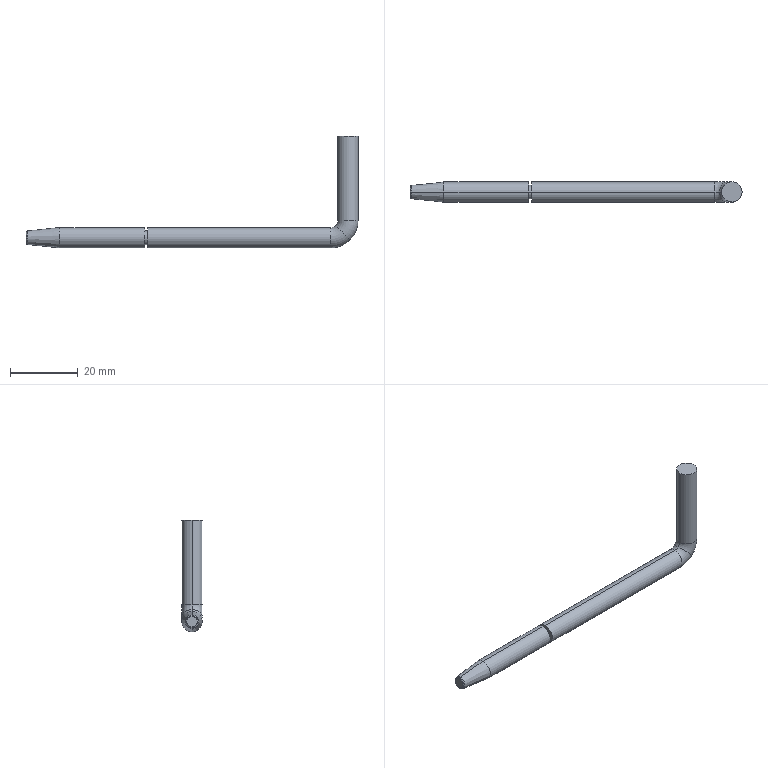Part | NX | features BREP 1 | 1 solid | 22 faces | box 98 x 6 x 33 mm | volume 3371 mm3 | cylinder 8 | torus 8 | plane 4 | cone 2 | commonest cylinder face diameters 6 x6 4 x2
STEP:
#1=CARTESIAN_POINT('',(90.,0.,-3.));
#2=VERTEX_POINT('',#1);
#3=CARTESIAN_POINT('',(35.9,0.,-3.));
#4=VERTEX_POINT('',#3);
#5=CARTESIAN_POINT('',(90.,0.,-3.));
#6=DIRECTION('',(-1.,0.,0.));
#7=VECTOR('',#6,1000.);
#8=LINE('',#5,#7);
#9=EDGE_CURVE('',#2,#4,#8,.T.);
#10=ORIENTED_EDGE('',*,*,#9,.T.);
#11=CARTESIAN_POINT('',(35.9,0.,3.));
#12=VERTEX_POINT('',#11);
#13=CARTESIAN_POINT('',(35.9,0.,0.));
#14=DIRECTION('',(1.,0.,0.));
#15=DIRECTION('',(0.,0.,-1.));
#16=AXIS2_PLACEMENT_3D('',#13,#14,#15);
#17=CIRCLE('',#16,3.);
#18=EDGE_CURVE('',#4,#12,#17,.T.);
#19=ORIENTED_EDGE('',*,*,#18,.T.);
#20=CARTESIAN_POINT('',(90.,0.,3.));
#21=VERTEX_POINT('',#20);
#22=CARTESIAN_POINT('',(90.,0.,3.));
#23=DIRECTION('',(-1.,0.,0.));
#24=VECTOR('',#23,1000.);
#25=LINE('',#22,#24);
#26=EDGE_CURVE('',#21,#12,#25,.T.);
#27=ORIENTED_EDGE('',*,*,#26,.F.);
#28=CARTESIAN_POINT('',(90.,0.,0.));
#29=DIRECTION('',(-1.,0.,0.));
#30=DIRECTION('',(0.,0.,1.));
#31=AXIS2_PLACEMENT_3D('',#28,#29,#30);
#32=CIRCLE('',#31,3.);
#33=EDGE_CURVE('',#21,#2,#32,.T.);
#34=ORIENTED_EDGE('',*,*,#33,.T.);
#35=EDGE_LOOP('',(#10,#19,#27,#34));
#36=FACE_BOUND('',#35,.T.);
#37=CARTESIAN_POINT('',(0.,0.,0.));
#38=DIRECTION('',(1.,0.,0.));
#39=DIRECTION('',(0.,0.,-1.));
#40=AXIS2_PLACEMENT_3D('',#37,#38,#39);
#41=CYLINDRICAL_SURFACE('',#40,3.);
#42=ADVANCED_FACE('',(#36),#41,.T.);
#43=CARTESIAN_POINT('',(91.414,0.,3.586));
#44=VERTEX_POINT('',#43);
#45=CARTESIAN_POINT('',(90.,0.,5.));
#46=DIRECTION('',(0.,1.,0.));
#47=DIRECTION('',(0.7071,0.,-0.7071));
#48=AXIS2_PLACEMENT_3D('',#45,#46,#47);
#49=CIRCLE('',#48,2.);
#50=EDGE_CURVE('',#21,#44,#49,.F.);
#51=ORIENTED_EDGE('',*,*,#50,.T.);
#52=CARTESIAN_POINT('',(95.657,0.,-0.6569));
#53=VERTEX_POINT('',#52);
#54=CARTESIAN_POINT('',(93.536,0.,1.464));
#55=DIRECTION('',(0.7071,0.,0.7071));
#56=DIRECTION('',(0.7071,0.,-0.7071));
#57=AXIS2_PLACEMENT_3D('',#54,#55,#56);
#58=CIRCLE('',#57,3.);
#59=EDGE_CURVE('',#53,#44,#58,.T.);
#60=ORIENTED_EDGE('',*,*,#59,.F.);
#61=CARTESIAN_POINT('',(90.,0.,5.));
#62=DIRECTION('',(0.,1.,0.));
#63=DIRECTION('',(0.7071,0.,-0.7071));
#64=AXIS2_PLACEMENT_3D('',#61,#62,#63);
#65=CIRCLE('',#64,8.);
#66=EDGE_CURVE('',#2,#53,#65,.F.);
#67=ORIENTED_EDGE('',*,*,#66,.F.);
#68=ORIENTED_EDGE('',*,*,#33,.F.);
#69=EDGE_LOOP('',(#51,#60,#67,#68));
#70=FACE_BOUND('',#69,.T.);
#71=CARTESIAN_POINT('',(90.,0.,5.));
#72=DIRECTION('',(0.,-1.,0.));
#73=DIRECTION('',(0.,0.,-1.));
#74=AXIS2_PLACEMENT_3D('',#71,#72,#73);
#75=TOROIDAL_SURFACE('',#74,5.,3.);
#76=ADVANCED_FACE('',(#70),#75,.T.);
#77=ORIENTED_EDGE('',*,*,#66,.T.);
#78=CARTESIAN_POINT('',(93.536,0.,1.464));
#79=DIRECTION('',(0.7071,0.,0.7071));
#80=DIRECTION('',(-0.7071,0.,0.7071));
#81=AXIS2_PLACEMENT_3D('',#78,#79,#80);
#82=CIRCLE('',#81,3.);
#83=EDGE_CURVE('',#44,#53,#82,.T.);
#84=ORIENTED_EDGE('',*,*,#83,.F.);
#85=ORIENTED_EDGE('',*,*,#50,.F.);
#86=CARTESIAN_POINT('',(90.,0.,0.));
#87=DIRECTION('',(-1.,0.,0.));
#88=DIRECTION('',(0.,0.,-1.));
#89=AXIS2_PLACEMENT_3D('',#86,#87,#88);
#90=CIRCLE('',#89,3.);
#91=EDGE_CURVE('',#2,#21,#90,.T.);
#92=ORIENTED_EDGE('',*,*,#91,.F.);
#93=EDGE_LOOP('',(#77,#84,#85,#92));
#94=FACE_BOUND('',#93,.T.);
#95=CARTESIAN_POINT('',(90.,0.,5.));
#96=DIRECTION('',(0.,-1.,0.));
#97=DIRECTION('',(0.,0.,-1.));
#98=AXIS2_PLACEMENT_3D('',#95,#96,#97);
#99=TOROIDAL_SURFACE('',#98,5.,3.);
#100=ADVANCED_FACE('',(#94),#99,.T.);
#101=ORIENTED_EDGE('',*,*,#26,.T.);
#102=CARTESIAN_POINT('',(35.9,0.,0.));
#103=DIRECTION('',(1.,0.,0.));
#104=DIRECTION('',(0.,0.,1.));
#105=AXIS2_PLACEMENT_3D('',#102,#103,#104);
#106=CIRCLE('',#105,3.);
#107=EDGE_CURVE('',#12,#4,#106,.T.);
#108=ORIENTED_EDGE('',*,*,#107,.T.);
#109=ORIENTED_EDGE('',*,*,#9,.F.);
#110=ORIENTED_EDGE('',*,*,#91,.T.);
#111=EDGE_LOOP('',(#101,#108,#109,#110));
#112=FACE_BOUND('',#111,.T.);
#113=CARTESIAN_POINT('',(0.,0.,0.));
#114=DIRECTION('',(1.,0.,0.));
#115=DIRECTION('',(0.,0.,-1.));
#116=AXIS2_PLACEMENT_3D('',#113,#114,#115);
#117=CYLINDRICAL_SURFACE('',#116,3.);
#118=ADVANCED_FACE('',(#112),#117,.T.);
#119=ORIENTED_EDGE('',*,*,#107,.F.);
#120=ORIENTED_EDGE('',*,*,#18,.F.);
#121=EDGE_LOOP('',(#119,#120));
#122=FACE_BOUND('',#121,.T.);
#123=CARTESIAN_POINT('',(35.9,0.,2.));
#124=VERTEX_POINT('',#123);
#125=CARTESIAN_POINT('',(35.9,0.,-2.));
#126=VERTEX_POINT('',#125);
#127=CARTESIAN_POINT('',(35.9,0.,0.));
#128=DIRECTION('',(-1.,0.,0.));
#129=DIRECTION('',(0.,0.,1.));
#130=AXIS2_PLACEMENT_3D('',#127,#128,#129);
#131=CIRCLE('',#130,2.);
#132=EDGE_CURVE('',#124,#126,#131,.T.);
#133=ORIENTED_EDGE('',*,*,#132,.F.);
#134=CARTESIAN_POINT('',(35.9,0.,0.));
#135=DIRECTION('',(-1.,0.,0.));
#136=DIRECTION('',(0.,0.,-1.));
#137=AXIS2_PLACEMENT_3D('',#134,#135,#136);
#138=CIRCLE('',#137,2.);
#139=EDGE_CURVE('',#126,#124,#138,.T.);
#140=ORIENTED_EDGE('',*,*,#139,.F.);
#141=EDGE_LOOP('',(#133,#140));
#142=FACE_BOUND('',#141,.T.);
#143=CARTESIAN_POINT('',(35.9,0.,0.));
#144=DIRECTION('',(-1.,0.,0.));
#145=DIRECTION('',(0.,0.,1.));
#146=AXIS2_PLACEMENT_3D('',#143,#144,#145);
#147=PLANE('',#146);
#148=ADVANCED_FACE('',(#122,#142),#147,.T.);
#149=CARTESIAN_POINT('',(35.,0.,2.));
#150=VERTEX_POINT('',#149);
#151=CARTESIAN_POINT('',(35.,0.,2.));
#152=DIRECTION('',(1.,0.,0.));
#153=VECTOR('',#152,1000.);
#154=LINE('',#151,#153);
#155=EDGE_CURVE('',#124,#150,#154,.F.);
#156=ORIENTED_EDGE('',*,*,#155,.T.);
#157=CARTESIAN_POINT('',(35.,0.,-2.));
#158=VERTEX_POINT('',#157);
#159=CARTESIAN_POINT('',(35.,0.,0.));
#160=DIRECTION('',(1.,0.,0.));
#161=DIRECTION('',(0.,0.,1.));
#162=AXIS2_PLACEMENT_3D('',#159,#160,#161);
#163=CIRCLE('',#162,2.);
#164=EDGE_CURVE('',#150,#158,#163,.T.);
#165=ORIENTED_EDGE('',*,*,#164,.T.);
#166=CARTESIAN_POINT('',(35.,0.,-2.));
#167=DIRECTION('',(1.,0.,0.));
#168=VECTOR('',#167,1000.);
#169=LINE('',#166,#168);
#170=EDGE_CURVE('',#126,#158,#169,.F.);
#171=ORIENTED_EDGE('',*,*,#170,.F.);
#172=ORIENTED_EDGE('',*,*,#139,.T.);
#173=EDGE_LOOP('',(#156,#165,#171,#172));
#174=FACE_BOUND('',#173,.T.);
#175=CARTESIAN_POINT('',(0.,0.,0.));
#176=DIRECTION('',(-1.,0.,0.));
#177=DIRECTION('',(0.,0.,1.));
#178=AXIS2_PLACEMENT_3D('',#175,#176,#177);
#179=CYLINDRICAL_SURFACE('',#178,2.);
#180=ADVANCED_FACE('',(#174),#179,.T.);
#181=ORIENTED_EDGE('',*,*,#170,.T.);
#182=CARTESIAN_POINT('',(35.,0.,0.));
#183=DIRECTION('',(1.,0.,0.));
#184=DIRECTION('',(0.,0.,-1.));
#185=AXIS2_PLACEMENT_3D('',#182,#183,#184);
#186=CIRCLE('',#185,2.);
#187=EDGE_CURVE('',#158,#150,#186,.T.);
#188=ORIENTED_EDGE('',*,*,#187,.T.);
#189=ORIENTED_EDGE('',*,*,#155,.F.);
#190=ORIENTED_EDGE('',*,*,#132,.T.);
#191=EDGE_LOOP('',(#181,#188,#189,#190));
#192=FACE_BOUND('',#191,.T.);
#193=CARTESIAN_POINT('',(0.,0.,0.));
#194=DIRECTION('',(-1.,0.,0.));
#195=DIRECTION('',(0.,0.,1.));
#196=AXIS2_PLACEMENT_3D('',#193,#194,#195);
#197=CYLINDRICAL_SURFACE('',#196,2.);
#198=ADVANCED_FACE('',(#192),#197,.T.);
#199=CARTESIAN_POINT('',(35.,0.,3.));
#200=VERTEX_POINT('',#199);
#201=CARTESIAN_POINT('',(35.,0.,-3.));
#202=VERTEX_POINT('',#201);
#203=CARTESIAN_POINT('',(35.,0.,0.));
#204=DIRECTION('',(-1.,0.,0.));
#205=DIRECTION('',(0.,0.,1.));
#206=AXIS2_PLACEMENT_3D('',#203,#204,#205);
#207=CIRCLE('',#206,3.);
#208=EDGE_CURVE('',#200,#202,#207,.T.);
#209=ORIENTED_EDGE('',*,*,#208,.F.);
#210=CARTESIAN_POINT('',(35.,0.,0.));
#211=DIRECTION('',(-1.,0.,0.));
#212=DIRECTION('',(0.,0.,-1.));
#213=AXIS2_PLACEMENT_3D('',#210,#211,#212);
#214=CIRCLE('',#213,3.);
#215=EDGE_CURVE('',#202,#200,#214,.T.);
#216=ORIENTED_EDGE('',*,*,#215,.F.);
#217=EDGE_LOOP('',(#209,#216));
#218=FACE_BOUND('',#217,.T.);
#219=ORIENTED_EDGE('',*,*,#164,.F.);
#220=ORIENTED_EDGE('',*,*,#187,.F.);
#221=EDGE_LOOP('',(#219,#220));
#222=FACE_BOUND('',#221,.T.);
#223=CARTESIAN_POINT('',(35.,0.,0.));
#224=DIRECTION('',(-1.,0.,0.));
#225=DIRECTION('',(0.,0.,1.));
#226=AXIS2_PLACEMENT_3D('',#223,#224,#225);
#227=PLANE('',#226);
#228=ADVANCED_FACE('',(#218,#222),#227,.F.);
#229=CARTESIAN_POINT('',(10.,0.,3.));
#230=VERTEX_POINT('',#229);
#231=CARTESIAN_POINT('',(35.,0.,3.));
#232=DIRECTION('',(-1.,0.,0.));
#233=VECTOR('',#232,1000.);
#234=LINE('',#231,#233);
#235=EDGE_CURVE('',#230,#200,#234,.F.);
#236=ORIENTED_EDGE('',*,*,#235,.F.);
#237=CARTESIAN_POINT('',(10.,0.,-3.));
#238=VERTEX_POINT('',#237);
#239=CARTESIAN_POINT('',(10.,0.,0.));
#240=DIRECTION('',(1.,0.,0.));
#241=DIRECTION('',(0.,0.,1.));
#242=AXIS2_PLACEMENT_3D('',#239,#240,#241);
#243=CIRCLE('',#242,3.);
#244=EDGE_CURVE('',#230,#238,#243,.T.);
#245=ORIENTED_EDGE('',*,*,#244,.T.);
#246=CARTESIAN_POINT('',(35.,0.,-3.));
#247=DIRECTION('',(-1.,0.,0.));
#248=VECTOR('',#247,1000.);
#249=LINE('',#246,#248);
#250=EDGE_CURVE('',#238,#202,#249,.F.);
#251=ORIENTED_EDGE('',*,*,#250,.T.);
#252=ORIENTED_EDGE('',*,*,#215,.T.);
#253=EDGE_LOOP('',(#236,#245,#251,#252));
#254=FACE_BOUND('',#253,.T.);
#255=CARTESIAN_POINT('',(0.,0.,0.));
#256=DIRECTION('',(1.,0.,0.));
#257=DIRECTION('',(0.,0.,-1.));
#258=AXIS2_PLACEMENT_3D('',#255,#256,#257);
#259=CYLINDRICAL_SURFACE('',#258,3.);
#260=ADVANCED_FACE('',(#254),#259,.T.);
#261=ORIENTED_EDGE('',*,*,#250,.F.);
#262=CARTESIAN_POINT('',(10.,0.,0.));
#263=DIRECTION('',(1.,0.,0.));
#264=DIRECTION('',(0.,0.,-1.));
#265=AXIS2_PLACEMENT_3D('',#262,#263,#264);
#266=CIRCLE('',#265,3.);
#267=EDGE_CURVE('',#238,#230,#266,.T.);
#268=ORIENTED_EDGE('',*,*,#267,.T.);
#269=ORIENTED_EDGE('',*,*,#235,.T.);
#270=ORIENTED_EDGE('',*,*,#208,.T.);
#271=EDGE_LOOP('',(#261,#268,#269,#270));
#272=FACE_BOUND('',#271,.T.);
#273=CARTESIAN_POINT('',(0.,0.,0.));
#274=DIRECTION('',(1.,0.,0.));
#275=DIRECTION('',(0.,0.,-1.));
#276=AXIS2_PLACEMENT_3D('',#273,#274,#275);
#277=CYLINDRICAL_SURFACE('',#276,3.);
#278=ADVANCED_FACE('',(#272),#277,.T.);
#279=CARTESIAN_POINT('',(0.4477,0.,1.996));
#280=VERTEX_POINT('',#279);
#281=CARTESIAN_POINT('',(10.,0.,3.));
#282=DIRECTION('',(-0.9945,0.,-0.1045));
#283=VECTOR('',#282,1000.);
#284=LINE('',#281,#283);
#285=EDGE_CURVE('',#280,#230,#284,.F.);
#286=ORIENTED_EDGE('',*,*,#285,.T.);
#287=ORIENTED_EDGE('',*,*,#267,.F.);
#288=CARTESIAN_POINT('',(0.4477,0.,-1.996));
#289=VERTEX_POINT('',#288);
#290=CARTESIAN_POINT('',(10.,0.,-3.));
#291=DIRECTION('',(-0.9945,0.,0.1045));
#292=VECTOR('',#291,1000.);
#293=LINE('',#290,#292);
#294=EDGE_CURVE('',#289,#238,#293,.F.);
#295=ORIENTED_EDGE('',*,*,#294,.F.);
#296=CARTESIAN_POINT('',(0.4477,0.,0.));
#297=DIRECTION('',(1.,0.,0.));
#298=DIRECTION('',(0.,0.,-1.));
#299=AXIS2_PLACEMENT_3D('',#296,#297,#298);
#300=CIRCLE('',#299,1.996);
#301=EDGE_CURVE('',#289,#280,#300,.T.);
#302=ORIENTED_EDGE('',*,*,#301,.T.);
#303=EDGE_LOOP('',(#286,#287,#295,#302));
#304=FACE_BOUND('',#303,.T.);
#305=CARTESIAN_POINT('',(5.224,0.,0.));
#306=DIRECTION('',(1.,0.,0.));
#307=DIRECTION('',(0.,0.,-1.));
#308=AXIS2_PLACEMENT_3D('',#305,#306,#307);
#309=CONICAL_SURFACE('',#308,2.498,0.1047);
#310=ADVANCED_FACE('',(#304),#309,.T.);
#311=CARTESIAN_POINT('',(0.1284,0.,-1.833));
#312=VERTEX_POINT('',#311);
#313=CARTESIAN_POINT('',(0.5,0.,-1.499));
#314=DIRECTION('',(0.,1.,0.));
#315=DIRECTION('',(-0.1045,0.,-0.9945));
#316=AXIS2_PLACEMENT_3D('',#313,#314,#315);
#317=CIRCLE('',#316,0.5);
#318=EDGE_CURVE('',#289,#312,#317,.T.);
#319=ORIENTED_EDGE('',*,*,#318,.T.);
#320=CARTESIAN_POINT('',(0.1284,0.,1.833));
#321=VERTEX_POINT('',#320);
#322=CARTESIAN_POINT('',(0.1284,0.,0.));
#323=DIRECTION('',(-1.,0.,0.));
#324=DIRECTION('',(0.,0.,1.));
#325=AXIS2_PLACEMENT_3D('',#322,#323,#324);
#326=CIRCLE('',#325,1.833);
#327=EDGE_CURVE('',#321,#312,#326,.T.);
#328=ORIENTED_EDGE('',*,*,#327,.F.);
#329=CARTESIAN_POINT('',(0.5,0.,1.499));
#330=DIRECTION('',(0.,-1.,0.));
#331=DIRECTION('',(-0.1045,0.,0.9945));
#332=AXIS2_PLACEMENT_3D('',#329,#330,#331);
#333=CIRCLE('',#332,0.5);
#334=EDGE_CURVE('',#280,#321,#333,.T.);
#335=ORIENTED_EDGE('',*,*,#334,.F.);
#336=ORIENTED_EDGE('',*,*,#301,.F.);
#337=EDGE_LOOP('',(#319,#328,#335,#336));
#338=FACE_BOUND('',#337,.T.);
#339=CARTESIAN_POINT('',(0.5,0.,0.));
#340=DIRECTION('',(1.,0.,0.));
#341=DIRECTION('',(0.,0.,-1.));
#342=AXIS2_PLACEMENT_3D('',#339,#340,#341);
#343=TOROIDAL_SURFACE('',#342,1.499,0.5);
#344=ADVANCED_FACE('',(#338),#343,.T.);
#345=ORIENTED_EDGE('',*,*,#334,.T.);
#346=CARTESIAN_POINT('',(0.1284,0.,0.));
#347=DIRECTION('',(-1.,0.,0.));
#348=DIRECTION('',(0.,0.,-1.));
#349=AXIS2_PLACEMENT_3D('',#346,#347,#348);
#350=CIRCLE('',#349,1.833);
#351=EDGE_CURVE('',#312,#321,#350,.T.);
#352=ORIENTED_EDGE('',*,*,#351,.F.);
#353=ORIENTED_EDGE('',*,*,#318,.F.);
#354=CARTESIAN_POINT('',(0.4477,0.,0.));
#355=DIRECTION('',(1.,0.,0.));
#356=DIRECTION('',(0.,0.,1.));
#357=AXIS2_PLACEMENT_3D('',#354,#355,#356);
#358=CIRCLE('',#357,1.996);
#359=EDGE_CURVE('',#280,#289,#358,.T.);
#360=ORIENTED_EDGE('',*,*,#359,.F.);
#361=EDGE_LOOP('',(#345,#352,#353,#360));
#362=FACE_BOUND('',#361,.T.);
#363=CARTESIAN_POINT('',(0.5,0.,0.));
#364=DIRECTION('',(1.,0.,0.));
#365=DIRECTION('',(0.,0.,-1.));
#366=AXIS2_PLACEMENT_3D('',#363,#364,#365);
#367=TOROIDAL_SURFACE('',#366,1.499,0.5);
#368=ADVANCED_FACE('',(#362),#367,.T.);
#369=ORIENTED_EDGE('',*,*,#294,.T.);
#370=ORIENTED_EDGE('',*,*,#244,.F.);
#371=ORIENTED_EDGE('',*,*,#285,.F.);
#372=ORIENTED_EDGE('',*,*,#359,.T.);
#373=EDGE_LOOP('',(#369,#370,#371,#372));
#374=FACE_BOUND('',#373,.T.);
#375=CARTESIAN_POINT('',(5.224,0.,0.));
#376=DIRECTION('',(1.,0.,0.));
#377=DIRECTION('',(0.,0.,-1.));
#378=AXIS2_PLACEMENT_3D('',#375,#376,#377);
#379=CONICAL_SURFACE('',#378,2.498,0.1047);
#380=ADVANCED_FACE('',(#374),#379,.T.);
#381=CARTESIAN_POINT('',(0.,0.,-1.499));
#382=VERTEX_POINT('',#381);
#383=CARTESIAN_POINT('',(0.5,0.,-1.499));
#384=DIRECTION('',(0.,1.,0.));
#385=DIRECTION('',(-0.7431,0.,-0.6691));
#386=AXIS2_PLACEMENT_3D('',#383,#384,#385);
#387=CIRCLE('',#386,0.5);
#388=EDGE_CURVE('',#312,#382,#387,.T.);
#389=ORIENTED_EDGE('',*,*,#388,.F.);
#390=ORIENTED_EDGE('',*,*,#351,.T.);
#391=CARTESIAN_POINT('',(0.,0.,1.499));
#392=VERTEX_POINT('',#391);
#393=CARTESIAN_POINT('',(0.5,0.,1.499));
#394=DIRECTION('',(0.,-1.,0.));
#395=DIRECTION('',(-0.7431,0.,0.6691));
#396=AXIS2_PLACEMENT_3D('',#393,#394,#395);
#397=CIRCLE('',#396,0.5);
#398=EDGE_CURVE('',#321,#392,#397,.T.);
#399=ORIENTED_EDGE('',*,*,#398,.T.);
#400=CARTESIAN_POINT('',(0.,0.,0.));
#401=DIRECTION('',(1.,0.,0.));
#402=DIRECTION('',(0.,0.,1.));
#403=AXIS2_PLACEMENT_3D('',#400,#401,#402);
#404=CIRCLE('',#403,1.499);
#405=EDGE_CURVE('',#392,#382,#404,.T.);
#406=ORIENTED_EDGE('',*,*,#405,.T.);
#407=EDGE_LOOP('',(#389,#390,#399,#406));
#408=FACE_BOUND('',#407,.T.);
#409=CARTESIAN_POINT('',(0.5,0.,0.));
#410=DIRECTION('',(1.,0.,0.));
#411=DIRECTION('',(0.,0.,-1.));
#412=AXIS2_PLACEMENT_3D('',#409,#410,#411);
#413=TOROIDAL_SURFACE('',#412,1.499,0.5);
#414=ADVANCED_FACE('',(#408),#413,.T.);
#415=CARTESIAN_POINT('',(0.,0.,0.));
#416=DIRECTION('',(1.,0.,0.));
#417=DIRECTION('',(0.,0.,-1.));
#418=AXIS2_PLACEMENT_3D('',#415,#416,#417);
#419=CIRCLE('',#418,1.499);
#420=EDGE_CURVE('',#382,#392,#419,.T.);
#421=ORIENTED_EDGE('',*,*,#420,.F.);
#422=ORIENTED_EDGE('',*,*,#405,.F.);
#423=EDGE_LOOP('',(#421,#422));
#424=FACE_BOUND('',#423,.T.);
#425=CARTESIAN_POINT('',(0.,0.,0.));
#426=DIRECTION('',(1.,0.,0.));
#427=DIRECTION('',(0.,1.,0.));
#428=AXIS2_PLACEMENT_3D('',#425,#426,#427);
#429=PLANE('',#428);
#430=ADVANCED_FACE('',(#424),#429,.F.);
#431=ORIENTED_EDGE('',*,*,#398,.F.);
#432=ORIENTED_EDGE('',*,*,#327,.T.);
#433=ORIENTED_EDGE('',*,*,#388,.T.);
#434=ORIENTED_EDGE('',*,*,#420,.T.);
#435=EDGE_LOOP('',(#431,#432,#433,#434));
#436=FACE_BOUND('',#435,.T.);
#437=CARTESIAN_POINT('',(0.5,0.,0.));
#438=DIRECTION('',(1.,0.,0.));
#439=DIRECTION('',(0.,0.,-1.));
#440=AXIS2_PLACEMENT_3D('',#437,#438,#439);
#441=TOROIDAL_SURFACE('',#440,1.499,0.5);
#442=ADVANCED_FACE('',(#436),#441,.T.);
#443=CARTESIAN_POINT('',(92.,0.,5.));
#444=VERTEX_POINT('',#443);
#445=CARTESIAN_POINT('',(90.,0.,5.));
#446=DIRECTION('',(0.,1.,0.));
#447=DIRECTION('',(1.,0.,0.));
#448=AXIS2_PLACEMENT_3D('',#445,#446,#447);
#449=CIRCLE('',#448,2.);
#450=EDGE_CURVE('',#444,#44,#449,.T.);
#451=ORIENTED_EDGE('',*,*,#450,.T.);
#452=ORIENTED_EDGE('',*,*,#83,.T.);
#453=CARTESIAN_POINT('',(98.,0.,5.));
#454=VERTEX_POINT('',#453);
#455=CARTESIAN_POINT('',(90.,0.,5.));
#456=DIRECTION('',(0.,1.,0.));
#457=DIRECTION('',(1.,0.,0.));
#458=AXIS2_PLACEMENT_3D('',#455,#456,#457);
#459=CIRCLE('',#458,8.);
#460=EDGE_CURVE('',#454,#53,#459,.T.);
#461=ORIENTED_EDGE('',*,*,#460,.F.);
#462=CARTESIAN_POINT('',(95.,0.,5.));
#463=DIRECTION('',(0.,0.,1.));
#464=DIRECTION('',(-1.,0.,0.));
#465=AXIS2_PLACEMENT_3D('',#462,#463,#464);
#466=CIRCLE('',#465,3.);
#467=EDGE_CURVE('',#444,#454,#466,.T.);
#468=ORIENTED_EDGE('',*,*,#467,.F.);
#469=EDGE_LOOP('',(#451,#452,#461,#468));
#470=FACE_BOUND('',#469,.T.);
#471=CARTESIAN_POINT('',(90.,0.,5.));
#472=DIRECTION('',(0.,-1.,0.));
#473=DIRECTION('',(0.,0.,-1.));
#474=AXIS2_PLACEMENT_3D('',#471,#472,#473);
#475=TOROIDAL_SURFACE('',#474,5.,3.);
#476=ADVANCED_FACE('',(#470),#475,.T.);
#477=CARTESIAN_POINT('',(92.,0.,30.));
#478=VERTEX_POINT('',#477);
#479=CARTESIAN_POINT('',(92.,0.,30.));
#480=DIRECTION('',(0.,0.,-1.));
#481=VECTOR('',#480,1000.);
#482=LINE('',#479,#481);
#483=EDGE_CURVE('',#478,#444,#482,.T.);
#484=ORIENTED_EDGE('',*,*,#483,.T.);
#485=ORIENTED_EDGE('',*,*,#467,.T.);
#486=CARTESIAN_POINT('',(98.,0.,30.));
#487=VERTEX_POINT('',#486);
#488=CARTESIAN_POINT('',(98.,0.,30.));
#489=DIRECTION('',(0.,0.,-1.));
#490=VECTOR('',#489,1000.);
#491=LINE('',#488,#490);
#492=EDGE_CURVE('',#487,#454,#491,.T.);
#493=ORIENTED_EDGE('',*,*,#492,.F.);
#494=CARTESIAN_POINT('',(95.,0.,30.));
#495=DIRECTION('',(0.,0.,-1.));
#496=DIRECTION('',(1.,0.,0.));
#497=AXIS2_PLACEMENT_3D('',#494,#495,#496);
#498=CIRCLE('',#497,3.);
#499=EDGE_CURVE('',#487,#478,#498,.T.);
#500=ORIENTED_EDGE('',*,*,#499,.T.);
#501=EDGE_LOOP('',(#484,#485,#493,#500));
#502=FACE_BOUND('',#501,.T.);
#503=CARTESIAN_POINT('',(95.,0.,5.));
#504=DIRECTION('',(0.,0.,1.));
#505=DIRECTION('',(1.,0.,0.));
#506=AXIS2_PLACEMENT_3D('',#503,#504,#505);
#507=CYLINDRICAL_SURFACE('',#506,3.);
#508=ADVANCED_FACE('',(#502),#507,.T.);
#509=ORIENTED_EDGE('',*,*,#499,.F.);
#510=CARTESIAN_POINT('',(95.,0.,30.));
#511=DIRECTION('',(0.,0.,-1.));
#512=DIRECTION('',(-1.,0.,0.));
#513=AXIS2_PLACEMENT_3D('',#510,#511,#512);
#514=CIRCLE('',#513,3.);
#515=EDGE_CURVE('',#478,#487,#514,.T.);
#516=ORIENTED_EDGE('',*,*,#515,.F.);
#517=EDGE_LOOP('',(#509,#516));
#518=FACE_BOUND('',#517,.T.);
#519=CARTESIAN_POINT('',(95.,0.,30.));
#520=DIRECTION('',(0.,0.,1.));
#521=DIRECTION('',(1.,0.,0.));
#522=AXIS2_PLACEMENT_3D('',#519,#520,#521);
#523=PLANE('',#522);
#524=ADVANCED_FACE('',(#518),#523,.T.);
#525=ORIENTED_EDGE('',*,*,#492,.T.);
#526=CARTESIAN_POINT('',(95.,0.,5.));
#527=DIRECTION('',(0.,0.,1.));
#528=DIRECTION('',(1.,0.,0.));
#529=AXIS2_PLACEMENT_3D('',#526,#527,#528);
#530=CIRCLE('',#529,3.);
#531=EDGE_CURVE('',#454,#444,#530,.T.);
#532=ORIENTED_EDGE('',*,*,#531,.T.);
#533=ORIENTED_EDGE('',*,*,#483,.F.);
#534=ORIENTED_EDGE('',*,*,#515,.T.);
#535=EDGE_LOOP('',(#525,#532,#533,#534));
#536=FACE_BOUND('',#535,.T.);
#537=CARTESIAN_POINT('',(95.,0.,5.));
#538=DIRECTION('',(0.,0.,1.));
#539=DIRECTION('',(1.,0.,0.));
#540=AXIS2_PLACEMENT_3D('',#537,#538,#539);
#541=CYLINDRICAL_SURFACE('',#540,3.);
#542=ADVANCED_FACE('',(#536),#541,.T.);
#543=ORIENTED_EDGE('',*,*,#460,.T.);
#544=ORIENTED_EDGE('',*,*,#59,.T.);
#545=ORIENTED_EDGE('',*,*,#450,.F.);
#546=ORIENTED_EDGE('',*,*,#531,.F.);
#547=EDGE_LOOP('',(#543,#544,#545,#546));
#548=FACE_BOUND('',#547,.T.);
#549=CARTESIAN_POINT('',(90.,0.,5.));
#550=DIRECTION('',(0.,-1.,0.));
#551=DIRECTION('',(0.,0.,-1.));
#552=AXIS2_PLACEMENT_3D('',#549,#550,#551);
#553=TOROIDAL_SURFACE('',#552,5.,3.);
#554=ADVANCED_FACE('',(#548),#553,.T.);
#555=CLOSED_SHELL('',(#42,#76,#100,#118,#148,#180,#198,#228,#260,#278,#310,#344,#368,#380,#414,#430,#442,#476,#508,#524,#542,#554));
#556=MANIFOLD_SOLID_BREP('',#555);
#557=(LENGTH_UNIT()NAMED_UNIT(*)SI_UNIT(.MILLI.,.METRE.));
#558=UNCERTAINTY_MEASURE_WITH_UNIT(LENGTH_MEASURE(0.00001),#557,'','');
#559=(NAMED_UNIT(*)PLANE_ANGLE_UNIT()SI_UNIT($,.RADIAN.));
#560=(NAMED_UNIT(*)SI_UNIT($,.STERADIAN.)SOLID_ANGLE_UNIT());
#561=(GEOMETRIC_REPRESENTATION_CONTEXT(3)GLOBAL_UNCERTAINTY_ASSIGNED_CONTEXT((#558))GLOBAL_UNIT_ASSIGNED_CONTEXT((#557,#559,#560))REPRESENTATION_CONTEXT('',''));
#562=ADVANCED_BREP_SHAPE_REPRESENTATION('',(#556),#561);